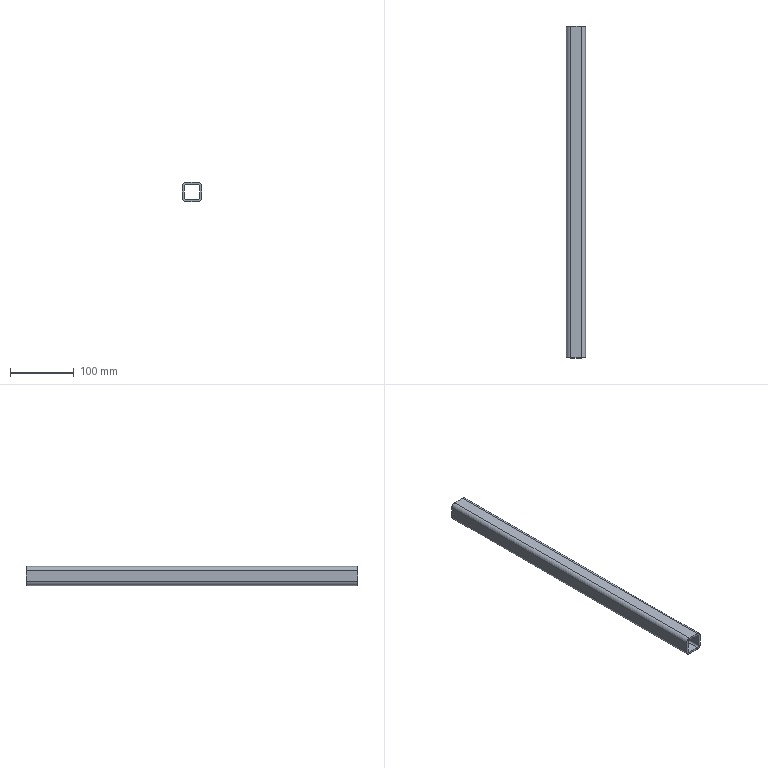Part | SolidWorks | features HoleWzd 1, ICE 1, WeldMemberFeat 1, WeldmentFeature 1 | 1 solid | 18 faces | box 30 x 520 x 30 mm | volume 164668 mm3 | plane 10 | cylinder 8 | commonest cylinder face diameters 6.4 x4 12.8 x4
STEP:
#1=CARTESIAN_POINT('',(-200.,260.,8.6));
#2=VERTEX_POINT('',#1);
#3=CARTESIAN_POINT('',(-206.4,260.,15.));
#4=VERTEX_POINT('',#3);
#5=CARTESIAN_POINT('',(-206.4,260.,8.6));
#6=DIRECTION('',(0.,-1.,0.));
#7=DIRECTION('',(1.,0.,0.));
#8=AXIS2_PLACEMENT_3D('',#5,#6,#7);
#9=CIRCLE('',#8,6.4);
#10=EDGE_CURVE('',#2,#4,#9,.T.);
#11=ORIENTED_EDGE('',*,*,#10,.T.);
#12=CARTESIAN_POINT('',(-206.4,-260.,15.));
#13=VERTEX_POINT('',#12);
#14=CARTESIAN_POINT('',(-206.4,-260.,15.));
#15=DIRECTION('',(0.,1.,0.));
#16=VECTOR('',#15,1000.);
#17=LINE('',#14,#16);
#18=EDGE_CURVE('',#13,#4,#17,.T.);
#19=ORIENTED_EDGE('',*,*,#18,.F.);
#20=CARTESIAN_POINT('',(-200.,-260.,8.6));
#21=VERTEX_POINT('',#20);
#22=CARTESIAN_POINT('',(-206.4,-260.,8.6));
#23=DIRECTION('',(0.,-1.,0.));
#24=DIRECTION('',(1.,0.,0.));
#25=AXIS2_PLACEMENT_3D('',#22,#23,#24);
#26=CIRCLE('',#25,6.4);
#27=EDGE_CURVE('',#21,#13,#26,.T.);
#28=ORIENTED_EDGE('',*,*,#27,.F.);
#29=CARTESIAN_POINT('',(-200.,-260.,8.6));
#30=DIRECTION('',(0.,1.,0.));
#31=VECTOR('',#30,1000.);
#32=LINE('',#29,#31);
#33=EDGE_CURVE('',#21,#2,#32,.T.);
#34=ORIENTED_EDGE('',*,*,#33,.T.);
#35=EDGE_LOOP('',(#11,#19,#28,#34));
#36=FACE_OUTER_BOUND('',#35,.T.);
#37=CARTESIAN_POINT('',(-206.4,-260.,8.6));
#38=DIRECTION('',(0.,1.,0.));
#39=DIRECTION('',(-1.,0.,0.));
#40=AXIS2_PLACEMENT_3D('',#37,#38,#39);
#41=CYLINDRICAL_SURFACE('',#40,6.4);
#42=ADVANCED_FACE('',(#36),#41,.T.);
#43=CARTESIAN_POINT('',(-223.6,260.,15.));
#44=VERTEX_POINT('',#43);
#45=CARTESIAN_POINT('',(-206.4,260.,15.));
#46=DIRECTION('',(-1.,0.,0.));
#47=VECTOR('',#46,1000.);
#48=LINE('',#45,#47);
#49=EDGE_CURVE('',#4,#44,#48,.T.);
#50=ORIENTED_EDGE('',*,*,#49,.T.);
#51=CARTESIAN_POINT('',(-223.6,-260.,15.));
#52=VERTEX_POINT('',#51);
#53=CARTESIAN_POINT('',(-223.6,-260.,15.));
#54=DIRECTION('',(0.,1.,0.));
#55=VECTOR('',#54,1000.);
#56=LINE('',#53,#55);
#57=EDGE_CURVE('',#52,#44,#56,.T.);
#58=ORIENTED_EDGE('',*,*,#57,.F.);
#59=CARTESIAN_POINT('',(-206.4,-260.,15.));
#60=DIRECTION('',(-1.,0.,0.));
#61=VECTOR('',#60,1000.);
#62=LINE('',#59,#61);
#63=EDGE_CURVE('',#13,#52,#62,.T.);
#64=ORIENTED_EDGE('',*,*,#63,.F.);
#65=ORIENTED_EDGE('',*,*,#18,.T.);
#66=EDGE_LOOP('',(#50,#58,#64,#65));
#67=FACE_OUTER_BOUND('',#66,.T.);
#68=CARTESIAN_POINT('',(-206.4,-260.,15.));
#69=DIRECTION('',(0.,0.,-1.));
#70=DIRECTION('',(-1.,0.,0.));
#71=AXIS2_PLACEMENT_3D('',#68,#69,#70);
#72=PLANE('',#71);
#73=ADVANCED_FACE('',(#67),#72,.F.);
#74=CARTESIAN_POINT('',(-230.,260.,8.6));
#75=VERTEX_POINT('',#74);
#76=CARTESIAN_POINT('',(-223.6,260.,8.6));
#77=DIRECTION('',(0.,-1.,0.));
#78=DIRECTION('',(1.,0.,0.));
#79=AXIS2_PLACEMENT_3D('',#76,#77,#78);
#80=CIRCLE('',#79,6.4);
#81=EDGE_CURVE('',#44,#75,#80,.T.);
#82=ORIENTED_EDGE('',*,*,#81,.T.);
#83=CARTESIAN_POINT('',(-230.,-260.,8.6));
#84=VERTEX_POINT('',#83);
#85=CARTESIAN_POINT('',(-230.,-260.,8.6));
#86=DIRECTION('',(0.,1.,0.));
#87=VECTOR('',#86,1000.);
#88=LINE('',#85,#87);
#89=EDGE_CURVE('',#84,#75,#88,.T.);
#90=ORIENTED_EDGE('',*,*,#89,.F.);
#91=CARTESIAN_POINT('',(-223.6,-260.,8.6));
#92=DIRECTION('',(0.,-1.,0.));
#93=DIRECTION('',(1.,0.,0.));
#94=AXIS2_PLACEMENT_3D('',#91,#92,#93);
#95=CIRCLE('',#94,6.4);
#96=EDGE_CURVE('',#52,#84,#95,.T.);
#97=ORIENTED_EDGE('',*,*,#96,.F.);
#98=ORIENTED_EDGE('',*,*,#57,.T.);
#99=EDGE_LOOP('',(#82,#90,#97,#98));
#100=FACE_OUTER_BOUND('',#99,.T.);
#101=CARTESIAN_POINT('',(-223.6,-260.,8.6));
#102=DIRECTION('',(0.,1.,0.));
#103=DIRECTION('',(-1.,0.,0.));
#104=AXIS2_PLACEMENT_3D('',#101,#102,#103);
#105=CYLINDRICAL_SURFACE('',#104,6.4);
#106=ADVANCED_FACE('',(#100),#105,.T.);
#107=CARTESIAN_POINT('',(-230.,260.,-8.6));
#108=VERTEX_POINT('',#107);
#109=CARTESIAN_POINT('',(-230.,260.,-8.6));
#110=DIRECTION('',(0.,0.,-1.));
#111=VECTOR('',#110,1000.);
#112=LINE('',#109,#111);
#113=EDGE_CURVE('',#75,#108,#112,.T.);
#114=ORIENTED_EDGE('',*,*,#113,.T.);
#115=CARTESIAN_POINT('',(-230.,-260.,-8.6));
#116=VERTEX_POINT('',#115);
#117=CARTESIAN_POINT('',(-230.,-260.,-8.6));
#118=DIRECTION('',(0.,1.,0.));
#119=VECTOR('',#118,1000.);
#120=LINE('',#117,#119);
#121=EDGE_CURVE('',#116,#108,#120,.T.);
#122=ORIENTED_EDGE('',*,*,#121,.F.);
#123=CARTESIAN_POINT('',(-230.,-260.,-8.6));
#124=DIRECTION('',(0.,0.,-1.));
#125=VECTOR('',#124,1000.);
#126=LINE('',#123,#125);
#127=EDGE_CURVE('',#84,#116,#126,.T.);
#128=ORIENTED_EDGE('',*,*,#127,.F.);
#129=ORIENTED_EDGE('',*,*,#89,.T.);
#130=EDGE_LOOP('',(#114,#122,#128,#129));
#131=FACE_OUTER_BOUND('',#130,.T.);
#132=CARTESIAN_POINT('',(-230.,-260.,-8.6));
#133=DIRECTION('',(1.,0.,0.));
#134=DIRECTION('',(0.,1.,0.));
#135=AXIS2_PLACEMENT_3D('',#132,#133,#134);
#136=PLANE('',#135);
#137=ADVANCED_FACE('',(#131),#136,.F.);
#138=CARTESIAN_POINT('',(-223.6,260.,-15.));
#139=VERTEX_POINT('',#138);
#140=CARTESIAN_POINT('',(-223.6,260.,-8.6));
#141=DIRECTION('',(0.,-1.,0.));
#142=DIRECTION('',(1.,0.,0.));
#143=AXIS2_PLACEMENT_3D('',#140,#141,#142);
#144=CIRCLE('',#143,6.4);
#145=EDGE_CURVE('',#108,#139,#144,.T.);
#146=ORIENTED_EDGE('',*,*,#145,.T.);
#147=CARTESIAN_POINT('',(-223.6,-260.,-15.));
#148=VERTEX_POINT('',#147);
#149=CARTESIAN_POINT('',(-223.6,-260.,-15.));
#150=DIRECTION('',(0.,1.,0.));
#151=VECTOR('',#150,1000.);
#152=LINE('',#149,#151);
#153=EDGE_CURVE('',#148,#139,#152,.T.);
#154=ORIENTED_EDGE('',*,*,#153,.F.);
#155=CARTESIAN_POINT('',(-223.6,-260.,-8.6));
#156=DIRECTION('',(0.,-1.,0.));
#157=DIRECTION('',(1.,0.,0.));
#158=AXIS2_PLACEMENT_3D('',#155,#156,#157);
#159=CIRCLE('',#158,6.4);
#160=EDGE_CURVE('',#116,#148,#159,.T.);
#161=ORIENTED_EDGE('',*,*,#160,.F.);
#162=ORIENTED_EDGE('',*,*,#121,.T.);
#163=EDGE_LOOP('',(#146,#154,#161,#162));
#164=FACE_OUTER_BOUND('',#163,.T.);
#165=CARTESIAN_POINT('',(-223.6,-260.,-8.6));
#166=DIRECTION('',(0.,1.,0.));
#167=DIRECTION('',(-1.,0.,0.));
#168=AXIS2_PLACEMENT_3D('',#165,#166,#167);
#169=CYLINDRICAL_SURFACE('',#168,6.4);
#170=ADVANCED_FACE('',(#164),#169,.T.);
#171=CARTESIAN_POINT('',(-206.4,260.,-15.));
#172=VERTEX_POINT('',#171);
#173=CARTESIAN_POINT('',(-223.6,260.,-15.));
#174=DIRECTION('',(1.,0.,0.));
#175=VECTOR('',#174,1000.);
#176=LINE('',#173,#175);
#177=EDGE_CURVE('',#139,#172,#176,.T.);
#178=ORIENTED_EDGE('',*,*,#177,.T.);
#179=CARTESIAN_POINT('',(-206.4,-260.,-15.));
#180=VERTEX_POINT('',#179);
#181=CARTESIAN_POINT('',(-206.4,-260.,-15.));
#182=DIRECTION('',(0.,1.,0.));
#183=VECTOR('',#182,1000.);
#184=LINE('',#181,#183);
#185=EDGE_CURVE('',#180,#172,#184,.T.);
#186=ORIENTED_EDGE('',*,*,#185,.F.);
#187=CARTESIAN_POINT('',(-223.6,-260.,-15.));
#188=DIRECTION('',(1.,0.,0.));
#189=VECTOR('',#188,1000.);
#190=LINE('',#187,#189);
#191=EDGE_CURVE('',#148,#180,#190,.T.);
#192=ORIENTED_EDGE('',*,*,#191,.F.);
#193=ORIENTED_EDGE('',*,*,#153,.T.);
#194=EDGE_LOOP('',(#178,#186,#192,#193));
#195=FACE_OUTER_BOUND('',#194,.T.);
#196=CARTESIAN_POINT('',(-223.6,-260.,-15.));
#197=DIRECTION('',(0.,0.,1.));
#198=DIRECTION('',(1.,0.,0.));
#199=AXIS2_PLACEMENT_3D('',#196,#197,#198);
#200=PLANE('',#199);
#201=ADVANCED_FACE('',(#195),#200,.F.);
#202=CARTESIAN_POINT('',(-200.,260.,-8.6));
#203=VERTEX_POINT('',#202);
#204=CARTESIAN_POINT('',(-206.4,260.,-8.6));
#205=DIRECTION('',(0.,-1.,0.));
#206=DIRECTION('',(1.,0.,0.));
#207=AXIS2_PLACEMENT_3D('',#204,#205,#206);
#208=CIRCLE('',#207,6.4);
#209=EDGE_CURVE('',#172,#203,#208,.T.);
#210=ORIENTED_EDGE('',*,*,#209,.T.);
#211=CARTESIAN_POINT('',(-200.,-260.,-8.6));
#212=VERTEX_POINT('',#211);
#213=CARTESIAN_POINT('',(-200.,-260.,-8.6));
#214=DIRECTION('',(0.,1.,0.));
#215=VECTOR('',#214,1000.);
#216=LINE('',#213,#215);
#217=EDGE_CURVE('',#212,#203,#216,.T.);
#218=ORIENTED_EDGE('',*,*,#217,.F.);
#219=CARTESIAN_POINT('',(-206.4,-260.,-8.6));
#220=DIRECTION('',(0.,-1.,0.));
#221=DIRECTION('',(1.,0.,0.));
#222=AXIS2_PLACEMENT_3D('',#219,#220,#221);
#223=CIRCLE('',#222,6.4);
#224=EDGE_CURVE('',#180,#212,#223,.T.);
#225=ORIENTED_EDGE('',*,*,#224,.F.);
#226=ORIENTED_EDGE('',*,*,#185,.T.);
#227=EDGE_LOOP('',(#210,#218,#225,#226));
#228=FACE_OUTER_BOUND('',#227,.T.);
#229=CARTESIAN_POINT('',(-206.4,-260.,-8.6));
#230=DIRECTION('',(0.,1.,0.));
#231=DIRECTION('',(-1.,0.,0.));
#232=AXIS2_PLACEMENT_3D('',#229,#230,#231);
#233=CYLINDRICAL_SURFACE('',#232,6.4);
#234=ADVANCED_FACE('',(#228),#233,.T.);
#235=CARTESIAN_POINT('',(-223.6,260.,11.8));
#236=VERTEX_POINT('',#235);
#237=CARTESIAN_POINT('',(-226.8,260.,8.6));
#238=VERTEX_POINT('',#237);
#239=CARTESIAN_POINT('',(-223.6,260.,8.6));
#240=DIRECTION('',(0.,-1.,0.));
#241=DIRECTION('',(1.,0.,0.));
#242=AXIS2_PLACEMENT_3D('',#239,#240,#241);
#243=CIRCLE('',#242,3.2);
#244=EDGE_CURVE('',#236,#238,#243,.T.);
#245=ORIENTED_EDGE('',*,*,#244,.F.);
#246=CARTESIAN_POINT('',(-223.6,-260.,11.8));
#247=VERTEX_POINT('',#246);
#248=CARTESIAN_POINT('',(-223.6,-260.,11.8));
#249=DIRECTION('',(0.,1.,0.));
#250=VECTOR('',#249,1000.);
#251=LINE('',#248,#250);
#252=EDGE_CURVE('',#247,#236,#251,.T.);
#253=ORIENTED_EDGE('',*,*,#252,.F.);
#254=CARTESIAN_POINT('',(-226.8,-260.,8.6));
#255=VERTEX_POINT('',#254);
#256=CARTESIAN_POINT('',(-223.6,-260.,8.6));
#257=DIRECTION('',(0.,-1.,0.));
#258=DIRECTION('',(1.,0.,0.));
#259=AXIS2_PLACEMENT_3D('',#256,#257,#258);
#260=CIRCLE('',#259,3.2);
#261=EDGE_CURVE('',#247,#255,#260,.T.);
#262=ORIENTED_EDGE('',*,*,#261,.T.);
#263=CARTESIAN_POINT('',(-226.8,-260.,8.6));
#264=DIRECTION('',(0.,1.,0.));
#265=VECTOR('',#264,1000.);
#266=LINE('',#263,#265);
#267=EDGE_CURVE('',#255,#238,#266,.T.);
#268=ORIENTED_EDGE('',*,*,#267,.T.);
#269=EDGE_LOOP('',(#245,#253,#262,#268));
#270=FACE_OUTER_BOUND('',#269,.T.);
#271=CARTESIAN_POINT('',(-223.6,-260.,8.6));
#272=DIRECTION('',(0.,1.,0.));
#273=DIRECTION('',(-1.,0.,0.));
#274=AXIS2_PLACEMENT_3D('',#271,#272,#273);
#275=CYLINDRICAL_SURFACE('',#274,3.2);
#276=ADVANCED_FACE('',(#270),#275,.F.);
#277=CARTESIAN_POINT('',(-206.4,260.,11.8));
#278=VERTEX_POINT('',#277);
#279=CARTESIAN_POINT('',(-206.4,260.,11.8));
#280=DIRECTION('',(-1.,0.,0.));
#281=VECTOR('',#280,1000.);
#282=LINE('',#279,#281);
#283=EDGE_CURVE('',#278,#236,#282,.T.);
#284=ORIENTED_EDGE('',*,*,#283,.F.);
#285=CARTESIAN_POINT('',(-206.4,-260.,11.8));
#286=VERTEX_POINT('',#285);
#287=CARTESIAN_POINT('',(-206.4,-260.,11.8));
#288=DIRECTION('',(0.,1.,0.));
#289=VECTOR('',#288,1000.);
#290=LINE('',#287,#289);
#291=EDGE_CURVE('',#286,#278,#290,.T.);
#292=ORIENTED_EDGE('',*,*,#291,.F.);
#293=CARTESIAN_POINT('',(-206.4,-260.,11.8));
#294=DIRECTION('',(-1.,0.,0.));
#295=VECTOR('',#294,1000.);
#296=LINE('',#293,#295);
#297=EDGE_CURVE('',#286,#247,#296,.T.);
#298=ORIENTED_EDGE('',*,*,#297,.T.);
#299=ORIENTED_EDGE('',*,*,#252,.T.);
#300=EDGE_LOOP('',(#284,#292,#298,#299));
#301=FACE_OUTER_BOUND('',#300,.T.);
#302=CARTESIAN_POINT('',(-206.4,-260.,11.8));
#303=DIRECTION('',(0.,0.,-1.));
#304=DIRECTION('',(-1.,0.,0.));
#305=AXIS2_PLACEMENT_3D('',#302,#303,#304);
#306=PLANE('',#305);
#307=ADVANCED_FACE('',(#301),#306,.T.);
#308=CARTESIAN_POINT('',(-203.2,260.,8.6));
#309=VERTEX_POINT('',#308);
#310=CARTESIAN_POINT('',(-206.4,260.,8.6));
#311=DIRECTION('',(0.,-1.,0.));
#312=DIRECTION('',(1.,0.,0.));
#313=AXIS2_PLACEMENT_3D('',#310,#311,#312);
#314=CIRCLE('',#313,3.2);
#315=EDGE_CURVE('',#309,#278,#314,.T.);
#316=ORIENTED_EDGE('',*,*,#315,.F.);
#317=CARTESIAN_POINT('',(-203.2,-260.,8.6));
#318=VERTEX_POINT('',#317);
#319=CARTESIAN_POINT('',(-203.2,-260.,8.6));
#320=DIRECTION('',(0.,1.,0.));
#321=VECTOR('',#320,1000.);
#322=LINE('',#319,#321);
#323=EDGE_CURVE('',#318,#309,#322,.T.);
#324=ORIENTED_EDGE('',*,*,#323,.F.);
#325=CARTESIAN_POINT('',(-206.4,-260.,8.6));
#326=DIRECTION('',(0.,-1.,0.));
#327=DIRECTION('',(1.,0.,0.));
#328=AXIS2_PLACEMENT_3D('',#325,#326,#327);
#329=CIRCLE('',#328,3.2);
#330=EDGE_CURVE('',#318,#286,#329,.T.);
#331=ORIENTED_EDGE('',*,*,#330,.T.);
#332=ORIENTED_EDGE('',*,*,#291,.T.);
#333=EDGE_LOOP('',(#316,#324,#331,#332));
#334=FACE_OUTER_BOUND('',#333,.T.);
#335=CARTESIAN_POINT('',(-206.4,-260.,8.6));
#336=DIRECTION('',(0.,1.,0.));
#337=DIRECTION('',(-1.,0.,0.));
#338=AXIS2_PLACEMENT_3D('',#335,#336,#337);
#339=CYLINDRICAL_SURFACE('',#338,3.2);
#340=ADVANCED_FACE('',(#334),#339,.F.);
#341=CARTESIAN_POINT('',(-203.2,260.,-8.6));
#342=VERTEX_POINT('',#341);
#343=CARTESIAN_POINT('',(-203.2,260.,8.6));
#344=DIRECTION('',(0.,0.,1.));
#345=VECTOR('',#344,1000.);
#346=LINE('',#343,#345);
#347=EDGE_CURVE('',#342,#309,#346,.T.);
#348=ORIENTED_EDGE('',*,*,#347,.F.);
#349=CARTESIAN_POINT('',(-203.2,-260.,-8.6));
#350=VERTEX_POINT('',#349);
#351=CARTESIAN_POINT('',(-203.2,-260.,-8.6));
#352=DIRECTION('',(0.,1.,0.));
#353=VECTOR('',#352,1000.);
#354=LINE('',#351,#353);
#355=EDGE_CURVE('',#350,#342,#354,.T.);
#356=ORIENTED_EDGE('',*,*,#355,.F.);
#357=CARTESIAN_POINT('',(-203.2,-260.,8.6));
#358=DIRECTION('',(0.,0.,1.));
#359=VECTOR('',#358,1000.);
#360=LINE('',#357,#359);
#361=EDGE_CURVE('',#350,#318,#360,.T.);
#362=ORIENTED_EDGE('',*,*,#361,.T.);
#363=ORIENTED_EDGE('',*,*,#323,.T.);
#364=EDGE_LOOP('',(#348,#356,#362,#363));
#365=FACE_OUTER_BOUND('',#364,.T.);
#366=CARTESIAN_POINT('',(-203.2,-260.,8.6));
#367=DIRECTION('',(-1.,0.,0.));
#368=DIRECTION('',(0.,-1.,0.));
#369=AXIS2_PLACEMENT_3D('',#366,#367,#368);
#370=PLANE('',#369);
#371=ADVANCED_FACE('',(#365),#370,.T.);
#372=CARTESIAN_POINT('',(-206.4,260.,-11.8));
#373=VERTEX_POINT('',#372);
#374=CARTESIAN_POINT('',(-206.4,260.,-8.6));
#375=DIRECTION('',(0.,-1.,0.));
#376=DIRECTION('',(1.,0.,0.));
#377=AXIS2_PLACEMENT_3D('',#374,#375,#376);
#378=CIRCLE('',#377,3.2);
#379=EDGE_CURVE('',#373,#342,#378,.T.);
#380=ORIENTED_EDGE('',*,*,#379,.F.);
#381=CARTESIAN_POINT('',(-206.4,-260.,-11.8));
#382=VERTEX_POINT('',#381);
#383=CARTESIAN_POINT('',(-206.4,-260.,-11.8));
#384=DIRECTION('',(0.,1.,0.));
#385=VECTOR('',#384,1000.);
#386=LINE('',#383,#385);
#387=EDGE_CURVE('',#382,#373,#386,.T.);
#388=ORIENTED_EDGE('',*,*,#387,.F.);
#389=CARTESIAN_POINT('',(-206.4,-260.,-8.6));
#390=DIRECTION('',(0.,-1.,0.));
#391=DIRECTION('',(1.,0.,0.));
#392=AXIS2_PLACEMENT_3D('',#389,#390,#391);
#393=CIRCLE('',#392,3.2);
#394=EDGE_CURVE('',#382,#350,#393,.T.);
#395=ORIENTED_EDGE('',*,*,#394,.T.);
#396=ORIENTED_EDGE('',*,*,#355,.T.);
#397=EDGE_LOOP('',(#380,#388,#395,#396));
#398=FACE_OUTER_BOUND('',#397,.T.);
#399=CARTESIAN_POINT('',(-206.4,-260.,-8.6));
#400=DIRECTION('',(0.,1.,0.));
#401=DIRECTION('',(-1.,0.,0.));
#402=AXIS2_PLACEMENT_3D('',#399,#400,#401);
#403=CYLINDRICAL_SURFACE('',#402,3.2);
#404=ADVANCED_FACE('',(#398),#403,.F.);
#405=CARTESIAN_POINT('',(-223.6,260.,-11.8));
#406=VERTEX_POINT('',#405);
#407=CARTESIAN_POINT('',(-223.6,260.,-11.8));
#408=DIRECTION('',(1.,0.,0.));
#409=VECTOR('',#408,1000.);
#410=LINE('',#407,#409);
#411=EDGE_CURVE('',#406,#373,#410,.T.);
#412=ORIENTED_EDGE('',*,*,#411,.F.);
#413=CARTESIAN_POINT('',(-223.6,-260.,-11.8));
#414=VERTEX_POINT('',#413);
#415=CARTESIAN_POINT('',(-223.6,-260.,-11.8));
#416=DIRECTION('',(0.,1.,0.));
#417=VECTOR('',#416,1000.);
#418=LINE('',#415,#417);
#419=EDGE_CURVE('',#414,#406,#418,.T.);
#420=ORIENTED_EDGE('',*,*,#419,.F.);
#421=CARTESIAN_POINT('',(-223.6,-260.,-11.8));
#422=DIRECTION('',(1.,0.,0.));
#423=VECTOR('',#422,1000.);
#424=LINE('',#421,#423);
#425=EDGE_CURVE('',#414,#382,#424,.T.);
#426=ORIENTED_EDGE('',*,*,#425,.T.);
#427=ORIENTED_EDGE('',*,*,#387,.T.);
#428=EDGE_LOOP('',(#412,#420,#426,#427));
#429=FACE_OUTER_BOUND('',#428,.T.);
#430=CARTESIAN_POINT('',(-223.6,-260.,-11.8));
#431=DIRECTION('',(0.,0.,1.));
#432=DIRECTION('',(1.,0.,0.));
#433=AXIS2_PLACEMENT_3D('',#430,#431,#432);
#434=PLANE('',#433);
#435=ADVANCED_FACE('',(#429),#434,.T.);
#436=CARTESIAN_POINT('',(-226.8,260.,-8.6));
#437=VERTEX_POINT('',#436);
#438=CARTESIAN_POINT('',(-223.6,260.,-8.6));
#439=DIRECTION('',(0.,-1.,0.));
#440=DIRECTION('',(1.,0.,0.));
#441=AXIS2_PLACEMENT_3D('',#438,#439,#440);
#442=CIRCLE('',#441,3.2);
#443=EDGE_CURVE('',#437,#406,#442,.T.);
#444=ORIENTED_EDGE('',*,*,#443,.F.);
#445=CARTESIAN_POINT('',(-226.8,-260.,-8.6));
#446=VERTEX_POINT('',#445);
#447=CARTESIAN_POINT('',(-226.8,-260.,-8.6));
#448=DIRECTION('',(0.,1.,0.));
#449=VECTOR('',#448,1000.);
#450=LINE('',#447,#449);
#451=EDGE_CURVE('',#446,#437,#450,.T.);
#452=ORIENTED_EDGE('',*,*,#451,.F.);
#453=CARTESIAN_POINT('',(-223.6,-260.,-8.6));
#454=DIRECTION('',(0.,-1.,0.));
#455=DIRECTION('',(1.,0.,0.));
#456=AXIS2_PLACEMENT_3D('',#453,#454,#455);
#457=CIRCLE('',#456,3.2);
#458=EDGE_CURVE('',#446,#414,#457,.T.);
#459=ORIENTED_EDGE('',*,*,#458,.T.);
#460=ORIENTED_EDGE('',*,*,#419,.T.);
#461=EDGE_LOOP('',(#444,#452,#459,#460));
#462=FACE_OUTER_BOUND('',#461,.T.);
#463=CARTESIAN_POINT('',(-223.6,-260.,-8.6));
#464=DIRECTION('',(0.,1.,0.));
#465=DIRECTION('',(-1.,0.,0.));
#466=AXIS2_PLACEMENT_3D('',#463,#464,#465);
#467=CYLINDRICAL_SURFACE('',#466,3.2);
#468=ADVANCED_FACE('',(#462),#467,.F.);
#469=CARTESIAN_POINT('',(-226.8,260.,-8.6));
#470=DIRECTION('',(0.,0.,-1.));
#471=VECTOR('',#470,1000.);
#472=LINE('',#469,#471);
#473=EDGE_CURVE('',#238,#437,#472,.T.);
#474=ORIENTED_EDGE('',*,*,#473,.F.);
#475=ORIENTED_EDGE('',*,*,#267,.F.);
#476=CARTESIAN_POINT('',(-226.8,-260.,-8.6));
#477=DIRECTION('',(0.,0.,-1.));
#478=VECTOR('',#477,1000.);
#479=LINE('',#476,#478);
#480=EDGE_CURVE('',#255,#446,#479,.T.);
#481=ORIENTED_EDGE('',*,*,#480,.T.);
#482=ORIENTED_EDGE('',*,*,#451,.T.);
#483=EDGE_LOOP('',(#474,#475,#481,#482));
#484=FACE_OUTER_BOUND('',#483,.T.);
#485=CARTESIAN_POINT('',(-226.8,-260.,-8.6));
#486=DIRECTION('',(1.,0.,0.));
#487=DIRECTION('',(0.,1.,0.));
#488=AXIS2_PLACEMENT_3D('',#485,#486,#487);
#489=PLANE('',#488);
#490=ADVANCED_FACE('',(#484),#489,.T.);
#491=CARTESIAN_POINT('',(-200.,260.,8.6));
#492=DIRECTION('',(0.,0.,1.));
#493=VECTOR('',#492,1000.);
#494=LINE('',#491,#493);
#495=EDGE_CURVE('',#203,#2,#494,.T.);
#496=ORIENTED_EDGE('',*,*,#495,.T.);
#497=ORIENTED_EDGE('',*,*,#33,.F.);
#498=CARTESIAN_POINT('',(-200.,-260.,8.6));
#499=DIRECTION('',(0.,0.,1.));
#500=VECTOR('',#499,1000.);
#501=LINE('',#498,#500);
#502=EDGE_CURVE('',#212,#21,#501,.T.);
#503=ORIENTED_EDGE('',*,*,#502,.F.);
#504=ORIENTED_EDGE('',*,*,#217,.T.);
#505=EDGE_LOOP('',(#496,#497,#503,#504));
#506=FACE_OUTER_BOUND('',#505,.T.);
#507=CARTESIAN_POINT('',(-200.,-260.,8.6));
#508=DIRECTION('',(-1.,0.,0.));
#509=DIRECTION('',(0.,-1.,0.));
#510=AXIS2_PLACEMENT_3D('',#507,#508,#509);
#511=PLANE('',#510);
#512=ADVANCED_FACE('',(#506),#511,.F.);
#513=ORIENTED_EDGE('',*,*,#261,.F.);
#514=ORIENTED_EDGE('',*,*,#297,.F.);
#515=ORIENTED_EDGE('',*,*,#330,.F.);
#516=ORIENTED_EDGE('',*,*,#361,.F.);
#517=ORIENTED_EDGE('',*,*,#394,.F.);
#518=ORIENTED_EDGE('',*,*,#425,.F.);
#519=ORIENTED_EDGE('',*,*,#458,.F.);
#520=ORIENTED_EDGE('',*,*,#480,.F.);
#521=EDGE_LOOP('',(#513,#514,#515,#516,#517,#518,#519,#520));
#522=FACE_BOUND('',#521,.T.);
#523=ORIENTED_EDGE('',*,*,#27,.T.);
#524=ORIENTED_EDGE('',*,*,#63,.T.);
#525=ORIENTED_EDGE('',*,*,#96,.T.);
#526=ORIENTED_EDGE('',*,*,#127,.T.);
#527=ORIENTED_EDGE('',*,*,#160,.T.);
#528=ORIENTED_EDGE('',*,*,#191,.T.);
#529=ORIENTED_EDGE('',*,*,#224,.T.);
#530=ORIENTED_EDGE('',*,*,#502,.T.);
#531=EDGE_LOOP('',(#523,#524,#525,#526,#527,#528,#529,#530));
#532=FACE_OUTER_BOUND('',#531,.T.);
#533=CARTESIAN_POINT('',(-206.4,-260.,8.6));
#534=DIRECTION('',(0.,-1.,0.));
#535=DIRECTION('',(1.,0.,0.));
#536=AXIS2_PLACEMENT_3D('',#533,#534,#535);
#537=PLANE('',#536);
#538=ADVANCED_FACE('',(#522,#532),#537,.T.);
#539=ORIENTED_EDGE('',*,*,#244,.T.);
#540=ORIENTED_EDGE('',*,*,#473,.T.);
#541=ORIENTED_EDGE('',*,*,#443,.T.);
#542=ORIENTED_EDGE('',*,*,#411,.T.);
#543=ORIENTED_EDGE('',*,*,#379,.T.);
#544=ORIENTED_EDGE('',*,*,#347,.T.);
#545=ORIENTED_EDGE('',*,*,#315,.T.);
#546=ORIENTED_EDGE('',*,*,#283,.T.);
#547=EDGE_LOOP('',(#539,#540,#541,#542,#543,#544,#545,#546));
#548=FACE_BOUND('',#547,.T.);
#549=ORIENTED_EDGE('',*,*,#10,.F.);
#550=ORIENTED_EDGE('',*,*,#495,.F.);
#551=ORIENTED_EDGE('',*,*,#209,.F.);
#552=ORIENTED_EDGE('',*,*,#177,.F.);
#553=ORIENTED_EDGE('',*,*,#145,.F.);
#554=ORIENTED_EDGE('',*,*,#113,.F.);
#555=ORIENTED_EDGE('',*,*,#81,.F.);
#556=ORIENTED_EDGE('',*,*,#49,.F.);
#557=EDGE_LOOP('',(#549,#550,#551,#552,#553,#554,#555,#556));
#558=FACE_OUTER_BOUND('',#557,.T.);
#559=CARTESIAN_POINT('',(-206.4,260.,8.6));
#560=DIRECTION('',(0.,-1.,0.));
#561=DIRECTION('',(1.,0.,0.));
#562=AXIS2_PLACEMENT_3D('',#559,#560,#561);
#563=PLANE('',#562);
#564=ADVANCED_FACE('',(#548,#558),#563,.F.);
#565=CLOSED_SHELL('',(#42,#73,#106,#137,#170,#201,#234,#276,#307,#340,#371,#404,#435,#468,#490,#512,#538,#564));
#566=MANIFOLD_SOLID_BREP('',#565);
#567=CARTESIAN_POINT('',(0.,0.,0.));
#568=DIRECTION('',(0.,0.,1.));
#569=DIRECTION('',(1.,0.,0.));
#570=AXIS2_PLACEMENT_3D('',#567,#568,#569);
#571=(LENGTH_UNIT()NAMED_UNIT(*)SI_UNIT(.MILLI.,.METRE.));
#572=UNCERTAINTY_MEASURE_WITH_UNIT(LENGTH_MEASURE(0.00001),#571,'','');
#573=(NAMED_UNIT(*)PLANE_ANGLE_UNIT()SI_UNIT($,.RADIAN.));
#574=(NAMED_UNIT(*)SI_UNIT($,.STERADIAN.)SOLID_ANGLE_UNIT());
#575=(GEOMETRIC_REPRESENTATION_CONTEXT(3)GLOBAL_UNCERTAINTY_ASSIGNED_CONTEXT((#572))GLOBAL_UNIT_ASSIGNED_CONTEXT((#571,#573,#574))REPRESENTATION_CONTEXT('',''));
#576=ADVANCED_BREP_SHAPE_REPRESENTATION('',(#566,#570),#575);